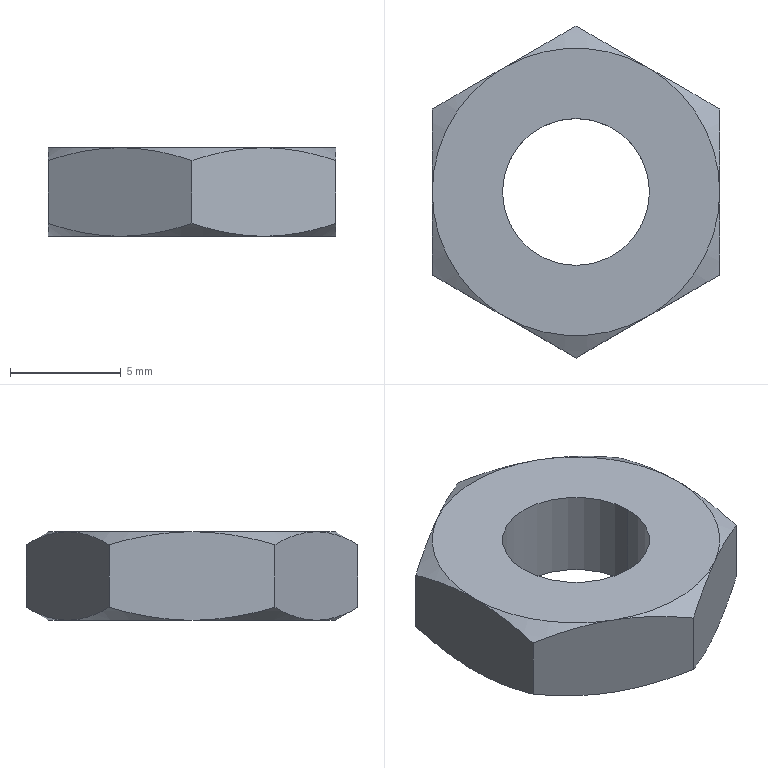Part | SolidWorks | features BaseBody 1 | 1 solid | 22 faces | box 13 x 15.011 x 4 mm | volume 441.798 mm3 | cone 12 | plane 8 | cylinder 2 | commonest cylinder face diameters 6.647 x2
STEP:
#1=CARTESIAN_POINT('',(-3.323,0.,4.));
#2=VERTEX_POINT('',#1);
#3=CARTESIAN_POINT('',(3.323,0.,4.));
#4=VERTEX_POINT('',#3);
#5=CARTESIAN_POINT('',(0.,0.,4.));
#6=DIRECTION('',(0.,0.,1.));
#7=DIRECTION('',(-1.,0.,0.));
#8=AXIS2_PLACEMENT_3D('',#5,#6,#7);
#9=CIRCLE('',#8,3.323);
#10=EDGE_CURVE('',#2,#4,#9,.T.);
#11=ORIENTED_EDGE('',*,*,#10,.T.);
#12=CARTESIAN_POINT('',(3.323,0.,0.));
#13=VERTEX_POINT('',#12);
#14=CARTESIAN_POINT('',(3.323,0.,4.));
#15=DIRECTION('',(0.,0.,-1.));
#16=VECTOR('',#15,1000.);
#17=LINE('',#14,#16);
#18=EDGE_CURVE('',#4,#13,#17,.T.);
#19=ORIENTED_EDGE('',*,*,#18,.T.);
#20=CARTESIAN_POINT('',(-3.323,0.,0.));
#21=VERTEX_POINT('',#20);
#22=CARTESIAN_POINT('',(0.,0.,0.));
#23=DIRECTION('',(0.,0.,1.));
#24=DIRECTION('',(-1.,0.,0.));
#25=AXIS2_PLACEMENT_3D('',#22,#23,#24);
#26=CIRCLE('',#25,3.323);
#27=EDGE_CURVE('',#21,#13,#26,.T.);
#28=ORIENTED_EDGE('',*,*,#27,.F.);
#29=CARTESIAN_POINT('',(-3.323,0.,4.));
#30=DIRECTION('',(0.,0.,-1.));
#31=VECTOR('',#30,1000.);
#32=LINE('',#29,#31);
#33=EDGE_CURVE('',#2,#21,#32,.T.);
#34=ORIENTED_EDGE('',*,*,#33,.F.);
#35=EDGE_LOOP('',(#11,#19,#28,#34));
#36=FACE_OUTER_BOUND('',#35,.T.);
#37=CARTESIAN_POINT('',(0.,0.,4.));
#38=DIRECTION('',(0.,0.,-1.));
#39=DIRECTION('',(-1.,0.,0.));
#40=AXIS2_PLACEMENT_3D('',#37,#38,#39);
#41=CYLINDRICAL_SURFACE('',#40,3.323);
#42=ADVANCED_FACE('',(#36),#41,.F.);
#43=CARTESIAN_POINT('',(-3.25,-5.629,4.));
#44=VERTEX_POINT('',#43);
#45=CARTESIAN_POINT('',(-6.5,0.,4.));
#46=VERTEX_POINT('',#45);
#47=CARTESIAN_POINT('',(0.,0.,4.));
#48=DIRECTION('',(0.,0.,-1.));
#49=DIRECTION('',(-1.,0.,0.));
#50=AXIS2_PLACEMENT_3D('',#47,#48,#49);
#51=CIRCLE('',#50,6.5);
#52=EDGE_CURVE('',#44,#46,#51,.T.);
#53=ORIENTED_EDGE('',*,*,#52,.F.);
#54=CARTESIAN_POINT('',(3.25,-5.629,4.));
#55=VERTEX_POINT('',#54);
#56=CARTESIAN_POINT('',(0.,0.,4.));
#57=DIRECTION('',(0.,0.,-1.));
#58=DIRECTION('',(-1.,0.,0.));
#59=AXIS2_PLACEMENT_3D('',#56,#57,#58);
#60=CIRCLE('',#59,6.5);
#61=EDGE_CURVE('',#55,#44,#60,.T.);
#62=ORIENTED_EDGE('',*,*,#61,.F.);
#63=CARTESIAN_POINT('',(6.5,0.,4.));
#64=VERTEX_POINT('',#63);
#65=CARTESIAN_POINT('',(0.,0.,4.));
#66=DIRECTION('',(0.,0.,-1.));
#67=DIRECTION('',(-1.,0.,0.));
#68=AXIS2_PLACEMENT_3D('',#65,#66,#67);
#69=CIRCLE('',#68,6.5);
#70=EDGE_CURVE('',#64,#55,#69,.T.);
#71=ORIENTED_EDGE('',*,*,#70,.F.);
#72=CARTESIAN_POINT('',(3.25,5.629,4.));
#73=VERTEX_POINT('',#72);
#74=CARTESIAN_POINT('',(0.,0.,4.));
#75=DIRECTION('',(0.,0.,-1.));
#76=DIRECTION('',(-1.,0.,0.));
#77=AXIS2_PLACEMENT_3D('',#74,#75,#76);
#78=CIRCLE('',#77,6.5);
#79=EDGE_CURVE('',#73,#64,#78,.T.);
#80=ORIENTED_EDGE('',*,*,#79,.F.);
#81=CARTESIAN_POINT('',(-3.25,5.629,4.));
#82=VERTEX_POINT('',#81);
#83=CARTESIAN_POINT('',(0.,0.,4.));
#84=DIRECTION('',(0.,0.,-1.));
#85=DIRECTION('',(-1.,0.,0.));
#86=AXIS2_PLACEMENT_3D('',#83,#84,#85);
#87=CIRCLE('',#86,6.5);
#88=EDGE_CURVE('',#82,#73,#87,.T.);
#89=ORIENTED_EDGE('',*,*,#88,.F.);
#90=CARTESIAN_POINT('',(0.,0.,4.));
#91=DIRECTION('',(0.,0.,-1.));
#92=DIRECTION('',(-1.,0.,0.));
#93=AXIS2_PLACEMENT_3D('',#90,#91,#92);
#94=CIRCLE('',#93,6.5);
#95=EDGE_CURVE('',#46,#82,#94,.T.);
#96=ORIENTED_EDGE('',*,*,#95,.F.);
#97=EDGE_LOOP('',(#53,#62,#71,#80,#89,#96));
#98=FACE_OUTER_BOUND('',#97,.T.);
#99=ORIENTED_EDGE('',*,*,#10,.F.);
#100=CARTESIAN_POINT('',(0.,0.,4.));
#101=DIRECTION('',(0.,0.,1.));
#102=DIRECTION('',(-1.,0.,0.));
#103=AXIS2_PLACEMENT_3D('',#100,#101,#102);
#104=CIRCLE('',#103,3.323);
#105=EDGE_CURVE('',#4,#2,#104,.T.);
#106=ORIENTED_EDGE('',*,*,#105,.F.);
#107=EDGE_LOOP('',(#99,#106));
#108=FACE_BOUND('',#107,.T.);
#109=CARTESIAN_POINT('',(6.5,3.753,4.));
#110=DIRECTION('',(0.,0.,-1.));
#111=DIRECTION('',(-1.,0.,0.));
#112=AXIS2_PLACEMENT_3D('',#109,#110,#111);
#113=PLANE('',#112);
#114=ADVANCED_FACE('',(#98,#108),#113,.F.);
#115=CARTESIAN_POINT('',(-6.5,3.753,3.419));
#116=VERTEX_POINT('',#115);
#117=CARTESIAN_POINT('',(-6.5,3.753,3.419));
#118=CARTESIAN_POINT('',(-6.5,2.527,3.773));
#119=CARTESIAN_POINT('',(-6.5,1.281,4.));
#120=CARTESIAN_POINT('',(-6.5,0.,4.));
#121=B_SPLINE_CURVE_WITH_KNOTS('',3,(#117,#118,#119,#120),.UNSPECIFIED.,.F.,.F.,(4,4),(0.,0.003797),.UNSPECIFIED.);
#122=EDGE_CURVE('',#116,#46,#121,.T.);
#123=ORIENTED_EDGE('',*,*,#122,.T.);
#124=ORIENTED_EDGE('',*,*,#95,.T.);
#125=CARTESIAN_POINT('',(-3.25,5.629,4.));
#126=CARTESIAN_POINT('',(-4.359,4.989,4.));
#127=CARTESIAN_POINT('',(-5.438,4.366,3.773));
#128=CARTESIAN_POINT('',(-6.5,3.753,3.419));
#129=B_SPLINE_CURVE_WITH_KNOTS('',3,(#125,#126,#127,#128),.UNSPECIFIED.,.F.,.F.,(4,4),(0.,0.003797),.UNSPECIFIED.);
#130=EDGE_CURVE('',#82,#116,#129,.T.);
#131=ORIENTED_EDGE('',*,*,#130,.T.);
#132=EDGE_LOOP('',(#123,#124,#131));
#133=FACE_OUTER_BOUND('',#132,.T.);
#134=CARTESIAN_POINT('',(0.,0.,3.416));
#135=DIRECTION('',(0.,0.,-1.));
#136=DIRECTION('',(-1.,0.,0.));
#137=AXIS2_PLACEMENT_3D('',#134,#135,#136);
#138=CONICAL_SURFACE('',#137,7.512,1.047);
#139=ADVANCED_FACE('',(#133),#138,.T.);
#140=CARTESIAN_POINT('',(-6.5,-3.753,3.419));
#141=VERTEX_POINT('',#140);
#142=CARTESIAN_POINT('',(-6.5,-3.753,3.419));
#143=CARTESIAN_POINT('',(-5.438,-4.366,3.773));
#144=CARTESIAN_POINT('',(-4.359,-4.989,4.));
#145=CARTESIAN_POINT('',(-3.25,-5.629,4.));
#146=B_SPLINE_CURVE_WITH_KNOTS('',3,(#142,#143,#144,#145),.UNSPECIFIED.,.F.,.F.,(4,4),(0.,0.003797),.UNSPECIFIED.);
#147=EDGE_CURVE('',#141,#44,#146,.T.);
#148=ORIENTED_EDGE('',*,*,#147,.T.);
#149=ORIENTED_EDGE('',*,*,#52,.T.);
#150=CARTESIAN_POINT('',(-6.5,0.,4.));
#151=CARTESIAN_POINT('',(-6.5,-1.281,4.));
#152=CARTESIAN_POINT('',(-6.5,-2.527,3.773));
#153=CARTESIAN_POINT('',(-6.5,-3.753,3.419));
#154=B_SPLINE_CURVE_WITH_KNOTS('',3,(#150,#151,#152,#153),.UNSPECIFIED.,.F.,.F.,(4,4),(0.,0.003797),.UNSPECIFIED.);
#155=EDGE_CURVE('',#46,#141,#154,.T.);
#156=ORIENTED_EDGE('',*,*,#155,.T.);
#157=EDGE_LOOP('',(#148,#149,#156));
#158=FACE_OUTER_BOUND('',#157,.T.);
#159=CARTESIAN_POINT('',(0.,0.,3.416));
#160=DIRECTION('',(0.,0.,-1.));
#161=DIRECTION('',(-1.,0.,0.));
#162=AXIS2_PLACEMENT_3D('',#159,#160,#161);
#163=CONICAL_SURFACE('',#162,7.512,1.047);
#164=ADVANCED_FACE('',(#158),#163,.T.);
#165=CARTESIAN_POINT('',(-0.000000043,-7.506,3.419));
#166=VERTEX_POINT('',#165);
#167=CARTESIAN_POINT('',(-0.000000043,-7.506,3.419));
#168=CARTESIAN_POINT('',(1.062,-6.892,3.773));
#169=CARTESIAN_POINT('',(2.141,-6.27,4.));
#170=CARTESIAN_POINT('',(3.25,-5.629,4.));
#171=B_SPLINE_CURVE_WITH_KNOTS('',3,(#167,#168,#169,#170),.UNSPECIFIED.,.F.,.F.,(4,4),(0.,0.003797),.UNSPECIFIED.);
#172=EDGE_CURVE('',#166,#55,#171,.T.);
#173=ORIENTED_EDGE('',*,*,#172,.T.);
#174=ORIENTED_EDGE('',*,*,#61,.T.);
#175=CARTESIAN_POINT('',(-3.25,-5.629,4.));
#176=CARTESIAN_POINT('',(-2.141,-6.27,4.));
#177=CARTESIAN_POINT('',(-1.062,-6.892,3.773));
#178=CARTESIAN_POINT('',(-0.000000043,-7.506,3.419));
#179=B_SPLINE_CURVE_WITH_KNOTS('',3,(#175,#176,#177,#178),.UNSPECIFIED.,.F.,.F.,(4,4),(0.,0.003797),.UNSPECIFIED.);
#180=EDGE_CURVE('',#44,#166,#179,.T.);
#181=ORIENTED_EDGE('',*,*,#180,.T.);
#182=EDGE_LOOP('',(#173,#174,#181));
#183=FACE_OUTER_BOUND('',#182,.T.);
#184=CARTESIAN_POINT('',(0.,0.,3.416));
#185=DIRECTION('',(0.,0.,-1.));
#186=DIRECTION('',(-1.,0.,0.));
#187=AXIS2_PLACEMENT_3D('',#184,#185,#186);
#188=CONICAL_SURFACE('',#187,7.512,1.047);
#189=ADVANCED_FACE('',(#183),#188,.T.);
#190=CARTESIAN_POINT('',(6.5,-3.753,3.419));
#191=VERTEX_POINT('',#190);
#192=CARTESIAN_POINT('',(6.5,-3.753,3.419));
#193=CARTESIAN_POINT('',(6.5,-2.527,3.773));
#194=CARTESIAN_POINT('',(6.5,-1.281,4.));
#195=CARTESIAN_POINT('',(6.5,0.,4.));
#196=B_SPLINE_CURVE_WITH_KNOTS('',3,(#192,#193,#194,#195),.UNSPECIFIED.,.F.,.F.,(4,4),(0.,0.003797),.UNSPECIFIED.);
#197=EDGE_CURVE('',#191,#64,#196,.T.);
#198=ORIENTED_EDGE('',*,*,#197,.T.);
#199=ORIENTED_EDGE('',*,*,#70,.T.);
#200=CARTESIAN_POINT('',(3.25,-5.629,4.));
#201=CARTESIAN_POINT('',(4.359,-4.989,4.));
#202=CARTESIAN_POINT('',(5.438,-4.366,3.773));
#203=CARTESIAN_POINT('',(6.5,-3.753,3.419));
#204=B_SPLINE_CURVE_WITH_KNOTS('',3,(#200,#201,#202,#203),.UNSPECIFIED.,.F.,.F.,(4,4),(0.,0.003797),.UNSPECIFIED.);
#205=EDGE_CURVE('',#55,#191,#204,.T.);
#206=ORIENTED_EDGE('',*,*,#205,.T.);
#207=EDGE_LOOP('',(#198,#199,#206));
#208=FACE_OUTER_BOUND('',#207,.T.);
#209=CARTESIAN_POINT('',(0.,0.,3.416));
#210=DIRECTION('',(0.,0.,-1.));
#211=DIRECTION('',(-1.,0.,0.));
#212=AXIS2_PLACEMENT_3D('',#209,#210,#211);
#213=CONICAL_SURFACE('',#212,7.512,1.047);
#214=ADVANCED_FACE('',(#208),#213,.T.);
#215=ORIENTED_EDGE('',*,*,#79,.T.);
#216=CARTESIAN_POINT('',(6.5,3.753,3.419));
#217=VERTEX_POINT('',#216);
#218=CARTESIAN_POINT('',(6.5,0.,4.));
#219=CARTESIAN_POINT('',(6.5,1.281,4.));
#220=CARTESIAN_POINT('',(6.5,2.527,3.773));
#221=CARTESIAN_POINT('',(6.5,3.753,3.419));
#222=B_SPLINE_CURVE_WITH_KNOTS('',3,(#218,#219,#220,#221),.UNSPECIFIED.,.F.,.F.,(4,4),(0.,0.003797),.UNSPECIFIED.);
#223=EDGE_CURVE('',#64,#217,#222,.T.);
#224=ORIENTED_EDGE('',*,*,#223,.T.);
#225=CARTESIAN_POINT('',(6.5,3.753,3.419));
#226=CARTESIAN_POINT('',(5.438,4.366,3.773));
#227=CARTESIAN_POINT('',(4.359,4.989,4.));
#228=CARTESIAN_POINT('',(3.25,5.629,4.));
#229=B_SPLINE_CURVE_WITH_KNOTS('',3,(#225,#226,#227,#228),.UNSPECIFIED.,.F.,.F.,(4,4),(0.,0.003797),.UNSPECIFIED.);
#230=EDGE_CURVE('',#217,#73,#229,.T.);
#231=ORIENTED_EDGE('',*,*,#230,.T.);
#232=EDGE_LOOP('',(#215,#224,#231));
#233=FACE_OUTER_BOUND('',#232,.T.);
#234=CARTESIAN_POINT('',(0.,0.,3.416));
#235=DIRECTION('',(0.,0.,-1.));
#236=DIRECTION('',(-1.,0.,0.));
#237=AXIS2_PLACEMENT_3D('',#234,#235,#236);
#238=CONICAL_SURFACE('',#237,7.512,1.047);
#239=ADVANCED_FACE('',(#233),#238,.T.);
#240=CARTESIAN_POINT('',(0.000000043,7.506,3.419));
#241=VERTEX_POINT('',#240);
#242=CARTESIAN_POINT('',(0.000000043,7.506,3.419));
#243=CARTESIAN_POINT('',(-1.062,6.892,3.773));
#244=CARTESIAN_POINT('',(-2.141,6.27,4.));
#245=CARTESIAN_POINT('',(-3.25,5.629,4.));
#246=B_SPLINE_CURVE_WITH_KNOTS('',3,(#242,#243,#244,#245),.UNSPECIFIED.,.F.,.F.,(4,4),(0.,0.003797),.UNSPECIFIED.);
#247=EDGE_CURVE('',#241,#82,#246,.T.);
#248=ORIENTED_EDGE('',*,*,#247,.T.);
#249=ORIENTED_EDGE('',*,*,#88,.T.);
#250=CARTESIAN_POINT('',(3.25,5.629,4.));
#251=CARTESIAN_POINT('',(2.141,6.27,4.));
#252=CARTESIAN_POINT('',(1.062,6.892,3.773));
#253=CARTESIAN_POINT('',(0.000000043,7.506,3.419));
#254=B_SPLINE_CURVE_WITH_KNOTS('',3,(#250,#251,#252,#253),.UNSPECIFIED.,.F.,.F.,(4,4),(0.,0.003797),.UNSPECIFIED.);
#255=EDGE_CURVE('',#73,#241,#254,.T.);
#256=ORIENTED_EDGE('',*,*,#255,.T.);
#257=EDGE_LOOP('',(#248,#249,#256));
#258=FACE_OUTER_BOUND('',#257,.T.);
#259=CARTESIAN_POINT('',(0.,0.,3.416));
#260=DIRECTION('',(0.,0.,-1.));
#261=DIRECTION('',(-1.,0.,0.));
#262=AXIS2_PLACEMENT_3D('',#259,#260,#261);
#263=CONICAL_SURFACE('',#262,7.512,1.047);
#264=ADVANCED_FACE('',(#258),#263,.T.);
#265=ORIENTED_EDGE('',*,*,#18,.F.);
#266=ORIENTED_EDGE('',*,*,#105,.T.);
#267=ORIENTED_EDGE('',*,*,#33,.T.);
#268=CARTESIAN_POINT('',(0.,0.,0.));
#269=DIRECTION('',(0.,0.,1.));
#270=DIRECTION('',(-1.,0.,0.));
#271=AXIS2_PLACEMENT_3D('',#268,#269,#270);
#272=CIRCLE('',#271,3.323);
#273=EDGE_CURVE('',#13,#21,#272,.T.);
#274=ORIENTED_EDGE('',*,*,#273,.F.);
#275=EDGE_LOOP('',(#265,#266,#267,#274));
#276=FACE_OUTER_BOUND('',#275,.T.);
#277=CARTESIAN_POINT('',(0.,0.,4.));
#278=DIRECTION('',(0.,0.,-1.));
#279=DIRECTION('',(-1.,0.,0.));
#280=AXIS2_PLACEMENT_3D('',#277,#278,#279);
#281=CYLINDRICAL_SURFACE('',#280,3.323);
#282=ADVANCED_FACE('',(#276),#281,.F.);
#283=CARTESIAN_POINT('',(-6.5,3.753,0.5806));
#284=VERTEX_POINT('',#283);
#285=CARTESIAN_POINT('',(-6.5,3.753,4.));
#286=DIRECTION('',(0.,0.,1.));
#287=VECTOR('',#286,1000.);
#288=LINE('',#285,#287);
#289=EDGE_CURVE('',#284,#116,#288,.T.);
#290=ORIENTED_EDGE('',*,*,#289,.F.);
#291=CARTESIAN_POINT('',(-6.5,0.,0.));
#292=VERTEX_POINT('',#291);
#293=CARTESIAN_POINT('',(-6.5,0.,0.));
#294=CARTESIAN_POINT('',(-6.5,1.281,0.));
#295=CARTESIAN_POINT('',(-6.5,2.527,0.2266));
#296=CARTESIAN_POINT('',(-6.5,3.753,0.5806));
#297=B_SPLINE_CURVE_WITH_KNOTS('',3,(#293,#294,#295,#296),.UNSPECIFIED.,.F.,.F.,(4,4),(0.,0.003797),.UNSPECIFIED.);
#298=EDGE_CURVE('',#292,#284,#297,.T.);
#299=ORIENTED_EDGE('',*,*,#298,.F.);
#300=CARTESIAN_POINT('',(-6.5,-3.753,0.5806));
#301=VERTEX_POINT('',#300);
#302=CARTESIAN_POINT('',(-6.5,-3.753,0.5806));
#303=CARTESIAN_POINT('',(-6.5,-2.527,0.2266));
#304=CARTESIAN_POINT('',(-6.5,-1.281,0.));
#305=CARTESIAN_POINT('',(-6.5,0.,0.));
#306=B_SPLINE_CURVE_WITH_KNOTS('',3,(#302,#303,#304,#305),.UNSPECIFIED.,.F.,.F.,(4,4),(0.,0.003797),.UNSPECIFIED.);
#307=EDGE_CURVE('',#301,#292,#306,.T.);
#308=ORIENTED_EDGE('',*,*,#307,.F.);
#309=CARTESIAN_POINT('',(-6.5,-3.753,4.));
#310=DIRECTION('',(0.,0.,-1.));
#311=VECTOR('',#310,1000.);
#312=LINE('',#309,#311);
#313=EDGE_CURVE('',#141,#301,#312,.T.);
#314=ORIENTED_EDGE('',*,*,#313,.F.);
#315=ORIENTED_EDGE('',*,*,#155,.F.);
#316=ORIENTED_EDGE('',*,*,#122,.F.);
#317=EDGE_LOOP('',(#290,#299,#308,#314,#315,#316));
#318=FACE_OUTER_BOUND('',#317,.T.);
#319=CARTESIAN_POINT('',(-6.5,3.753,4.));
#320=DIRECTION('',(1.,0.,0.));
#321=DIRECTION('',(0.,1.,0.));
#322=AXIS2_PLACEMENT_3D('',#319,#320,#321);
#323=PLANE('',#322);
#324=ADVANCED_FACE('',(#318),#323,.F.);
#325=CARTESIAN_POINT('',(0.,7.506,0.5806));
#326=VERTEX_POINT('',#325);
#327=CARTESIAN_POINT('',(0.,7.506,4.));
#328=DIRECTION('',(0.,0.,1.));
#329=VECTOR('',#328,1000.);
#330=LINE('',#327,#329);
#331=EDGE_CURVE('',#326,#241,#330,.T.);
#332=ORIENTED_EDGE('',*,*,#331,.F.);
#333=CARTESIAN_POINT('',(-3.25,5.629,0.));
#334=VERTEX_POINT('',#333);
#335=CARTESIAN_POINT('',(-3.25,5.629,0.));
#336=CARTESIAN_POINT('',(-2.141,6.27,0.));
#337=CARTESIAN_POINT('',(-1.062,6.892,0.2266));
#338=CARTESIAN_POINT('',(0.,7.506,0.5806));
#339=B_SPLINE_CURVE_WITH_KNOTS('',3,(#335,#336,#337,#338),.UNSPECIFIED.,.F.,.F.,(4,4),(0.,0.003797),.UNSPECIFIED.);
#340=EDGE_CURVE('',#334,#326,#339,.T.);
#341=ORIENTED_EDGE('',*,*,#340,.F.);
#342=CARTESIAN_POINT('',(-6.5,3.753,0.5806));
#343=CARTESIAN_POINT('',(-5.438,4.366,0.2266));
#344=CARTESIAN_POINT('',(-4.359,4.989,0.));
#345=CARTESIAN_POINT('',(-3.25,5.629,0.));
#346=B_SPLINE_CURVE_WITH_KNOTS('',3,(#342,#343,#344,#345),.UNSPECIFIED.,.F.,.F.,(4,4),(0.,0.003797),.UNSPECIFIED.);
#347=EDGE_CURVE('',#284,#334,#346,.T.);
#348=ORIENTED_EDGE('',*,*,#347,.F.);
#349=ORIENTED_EDGE('',*,*,#289,.T.);
#350=ORIENTED_EDGE('',*,*,#130,.F.);
#351=ORIENTED_EDGE('',*,*,#247,.F.);
#352=EDGE_LOOP('',(#332,#341,#348,#349,#350,#351));
#353=FACE_OUTER_BOUND('',#352,.T.);
#354=CARTESIAN_POINT('',(0.,7.506,4.));
#355=DIRECTION('',(0.5,-0.866,0.));
#356=DIRECTION('',(0.866,0.5,0.));
#357=AXIS2_PLACEMENT_3D('',#354,#355,#356);
#358=PLANE('',#357);
#359=ADVANCED_FACE('',(#353),#358,.F.);
#360=ORIENTED_EDGE('',*,*,#313,.T.);
#361=CARTESIAN_POINT('',(-3.25,-5.629,0.));
#362=VERTEX_POINT('',#361);
#363=CARTESIAN_POINT('',(-3.25,-5.629,0.));
#364=CARTESIAN_POINT('',(-4.359,-4.989,0.));
#365=CARTESIAN_POINT('',(-5.438,-4.366,0.2266));
#366=CARTESIAN_POINT('',(-6.5,-3.753,0.5806));
#367=B_SPLINE_CURVE_WITH_KNOTS('',3,(#363,#364,#365,#366),.UNSPECIFIED.,.F.,.F.,(4,4),(0.,0.003797),.UNSPECIFIED.);
#368=EDGE_CURVE('',#362,#301,#367,.T.);
#369=ORIENTED_EDGE('',*,*,#368,.F.);
#370=CARTESIAN_POINT('',(0.,-7.506,0.5806));
#371=VERTEX_POINT('',#370);
#372=CARTESIAN_POINT('',(0.,-7.506,0.5806));
#373=CARTESIAN_POINT('',(-1.062,-6.892,0.2266));
#374=CARTESIAN_POINT('',(-2.141,-6.27,0.));
#375=CARTESIAN_POINT('',(-3.25,-5.629,0.));
#376=B_SPLINE_CURVE_WITH_KNOTS('',3,(#372,#373,#374,#375),.UNSPECIFIED.,.F.,.F.,(4,4),(0.,0.003797),.UNSPECIFIED.);
#377=EDGE_CURVE('',#371,#362,#376,.T.);
#378=ORIENTED_EDGE('',*,*,#377,.F.);
#379=CARTESIAN_POINT('',(0.,-7.506,4.));
#380=DIRECTION('',(0.,0.,-1.));
#381=VECTOR('',#380,1000.);
#382=LINE('',#379,#381);
#383=EDGE_CURVE('',#166,#371,#382,.T.);
#384=ORIENTED_EDGE('',*,*,#383,.F.);
#385=ORIENTED_EDGE('',*,*,#180,.F.);
#386=ORIENTED_EDGE('',*,*,#147,.F.);
#387=EDGE_LOOP('',(#360,#369,#378,#384,#385,#386));
#388=FACE_OUTER_BOUND('',#387,.T.);
#389=CARTESIAN_POINT('',(-6.5,-3.753,4.));
#390=DIRECTION('',(0.5,0.866,0.));
#391=DIRECTION('',(-0.866,0.5,0.));
#392=AXIS2_PLACEMENT_3D('',#389,#390,#391);
#393=PLANE('',#392);
#394=ADVANCED_FACE('',(#388),#393,.F.);
#395=ORIENTED_EDGE('',*,*,#383,.T.);
#396=CARTESIAN_POINT('',(3.25,-5.629,0.));
#397=VERTEX_POINT('',#396);
#398=CARTESIAN_POINT('',(3.25,-5.629,0.));
#399=CARTESIAN_POINT('',(2.141,-6.27,0.));
#400=CARTESIAN_POINT('',(1.062,-6.892,0.2266));
#401=CARTESIAN_POINT('',(0.,-7.506,0.5806));
#402=B_SPLINE_CURVE_WITH_KNOTS('',3,(#398,#399,#400,#401),.UNSPECIFIED.,.F.,.F.,(4,4),(0.,0.003797),.UNSPECIFIED.);
#403=EDGE_CURVE('',#397,#371,#402,.T.);
#404=ORIENTED_EDGE('',*,*,#403,.F.);
#405=CARTESIAN_POINT('',(6.5,-3.753,0.5806));
#406=VERTEX_POINT('',#405);
#407=CARTESIAN_POINT('',(6.5,-3.753,0.5806));
#408=CARTESIAN_POINT('',(5.438,-4.366,0.2266));
#409=CARTESIAN_POINT('',(4.359,-4.989,0.));
#410=CARTESIAN_POINT('',(3.25,-5.629,0.));
#411=B_SPLINE_CURVE_WITH_KNOTS('',3,(#407,#408,#409,#410),.UNSPECIFIED.,.F.,.F.,(4,4),(0.,0.003797),.UNSPECIFIED.);
#412=EDGE_CURVE('',#406,#397,#411,.T.);
#413=ORIENTED_EDGE('',*,*,#412,.F.);
#414=CARTESIAN_POINT('',(6.5,-3.753,4.));
#415=DIRECTION('',(0.,0.,-1.));
#416=VECTOR('',#415,1000.);
#417=LINE('',#414,#416);
#418=EDGE_CURVE('',#191,#406,#417,.T.);
#419=ORIENTED_EDGE('',*,*,#418,.F.);
#420=ORIENTED_EDGE('',*,*,#205,.F.);
#421=ORIENTED_EDGE('',*,*,#172,.F.);
#422=EDGE_LOOP('',(#395,#404,#413,#419,#420,#421));
#423=FACE_OUTER_BOUND('',#422,.T.);
#424=CARTESIAN_POINT('',(0.,-7.506,4.));
#425=DIRECTION('',(-0.5,0.866,0.));
#426=DIRECTION('',(-0.866,-0.5,0.));
#427=AXIS2_PLACEMENT_3D('',#424,#425,#426);
#428=PLANE('',#427);
#429=ADVANCED_FACE('',(#423),#428,.F.);
#430=ORIENTED_EDGE('',*,*,#418,.T.);
#431=CARTESIAN_POINT('',(6.5,0.,0.));
#432=VERTEX_POINT('',#431);
#433=CARTESIAN_POINT('',(6.5,0.,0.));
#434=CARTESIAN_POINT('',(6.5,-1.281,0.));
#435=CARTESIAN_POINT('',(6.5,-2.527,0.2266));
#436=CARTESIAN_POINT('',(6.5,-3.753,0.5806));
#437=B_SPLINE_CURVE_WITH_KNOTS('',3,(#433,#434,#435,#436),.UNSPECIFIED.,.F.,.F.,(4,4),(0.,0.003797),.UNSPECIFIED.);
#438=EDGE_CURVE('',#432,#406,#437,.T.);
#439=ORIENTED_EDGE('',*,*,#438,.F.);
#440=CARTESIAN_POINT('',(6.5,3.753,0.5806));
#441=VERTEX_POINT('',#440);
#442=CARTESIAN_POINT('',(6.5,3.753,0.5806));
#443=CARTESIAN_POINT('',(6.5,2.527,0.2266));
#444=CARTESIAN_POINT('',(6.5,1.281,0.));
#445=CARTESIAN_POINT('',(6.5,0.,0.));
#446=B_SPLINE_CURVE_WITH_KNOTS('',3,(#442,#443,#444,#445),.UNSPECIFIED.,.F.,.F.,(4,4),(0.,0.003797),.UNSPECIFIED.);
#447=EDGE_CURVE('',#441,#432,#446,.T.);
#448=ORIENTED_EDGE('',*,*,#447,.F.);
#449=CARTESIAN_POINT('',(6.5,3.753,4.));
#450=DIRECTION('',(0.,0.,-1.));
#451=VECTOR('',#450,1000.);
#452=LINE('',#449,#451);
#453=EDGE_CURVE('',#217,#441,#452,.T.);
#454=ORIENTED_EDGE('',*,*,#453,.F.);
#455=ORIENTED_EDGE('',*,*,#223,.F.);
#456=ORIENTED_EDGE('',*,*,#197,.F.);
#457=EDGE_LOOP('',(#430,#439,#448,#454,#455,#456));
#458=FACE_OUTER_BOUND('',#457,.T.);
#459=CARTESIAN_POINT('',(6.5,-3.753,4.));
#460=DIRECTION('',(-1.,0.,0.));
#461=DIRECTION('',(0.,-1.,0.));
#462=AXIS2_PLACEMENT_3D('',#459,#460,#461);
#463=PLANE('',#462);
#464=ADVANCED_FACE('',(#458),#463,.F.);
#465=ORIENTED_EDGE('',*,*,#453,.T.);
#466=CARTESIAN_POINT('',(3.25,5.629,0.));
#467=VERTEX_POINT('',#466);
#468=CARTESIAN_POINT('',(3.25,5.629,0.));
#469=CARTESIAN_POINT('',(4.359,4.989,0.));
#470=CARTESIAN_POINT('',(5.438,4.366,0.2266));
#471=CARTESIAN_POINT('',(6.5,3.753,0.5806));
#472=B_SPLINE_CURVE_WITH_KNOTS('',3,(#468,#469,#470,#471),.UNSPECIFIED.,.F.,.F.,(4,4),(0.,0.003797),.UNSPECIFIED.);
#473=EDGE_CURVE('',#467,#441,#472,.T.);
#474=ORIENTED_EDGE('',*,*,#473,.F.);
#475=CARTESIAN_POINT('',(0.,7.506,0.5806));
#476=CARTESIAN_POINT('',(1.062,6.892,0.2266));
#477=CARTESIAN_POINT('',(2.141,6.27,0.));
#478=CARTESIAN_POINT('',(3.25,5.629,0.));
#479=B_SPLINE_CURVE_WITH_KNOTS('',3,(#475,#476,#477,#478),.UNSPECIFIED.,.F.,.F.,(4,4),(0.,0.003797),.UNSPECIFIED.);
#480=EDGE_CURVE('',#326,#467,#479,.T.);
#481=ORIENTED_EDGE('',*,*,#480,.F.);
#482=ORIENTED_EDGE('',*,*,#331,.T.);
#483=ORIENTED_EDGE('',*,*,#255,.F.);
#484=ORIENTED_EDGE('',*,*,#230,.F.);
#485=EDGE_LOOP('',(#465,#474,#481,#482,#483,#484));
#486=FACE_OUTER_BOUND('',#485,.T.);
#487=CARTESIAN_POINT('',(6.5,3.753,4.));
#488=DIRECTION('',(-0.5,-0.866,0.));
#489=DIRECTION('',(0.866,-0.5,0.));
#490=AXIS2_PLACEMENT_3D('',#487,#488,#489);
#491=PLANE('',#490);
#492=ADVANCED_FACE('',(#486),#491,.F.);
#493=CARTESIAN_POINT('',(0.,0.,0.));
#494=DIRECTION('',(0.,0.,-1.));
#495=DIRECTION('',(1.,0.,0.));
#496=AXIS2_PLACEMENT_3D('',#493,#494,#495);
#497=CIRCLE('',#496,6.5);
#498=EDGE_CURVE('',#432,#397,#497,.T.);
#499=ORIENTED_EDGE('',*,*,#498,.T.);
#500=CARTESIAN_POINT('',(0.,0.,0.));
#501=DIRECTION('',(0.,0.,-1.));
#502=DIRECTION('',(1.,0.,0.));
#503=AXIS2_PLACEMENT_3D('',#500,#501,#502);
#504=CIRCLE('',#503,6.5);
#505=EDGE_CURVE('',#397,#362,#504,.T.);
#506=ORIENTED_EDGE('',*,*,#505,.T.);
#507=CARTESIAN_POINT('',(0.,0.,0.));
#508=DIRECTION('',(0.,0.,-1.));
#509=DIRECTION('',(1.,0.,0.));
#510=AXIS2_PLACEMENT_3D('',#507,#508,#509);
#511=CIRCLE('',#510,6.5);
#512=EDGE_CURVE('',#362,#292,#511,.T.);
#513=ORIENTED_EDGE('',*,*,#512,.T.);
#514=CARTESIAN_POINT('',(0.,0.,0.));
#515=DIRECTION('',(0.,0.,-1.));
#516=DIRECTION('',(1.,0.,0.));
#517=AXIS2_PLACEMENT_3D('',#514,#515,#516);
#518=CIRCLE('',#517,6.5);
#519=EDGE_CURVE('',#292,#334,#518,.T.);
#520=ORIENTED_EDGE('',*,*,#519,.T.);
#521=CARTESIAN_POINT('',(0.,0.,0.));
#522=DIRECTION('',(0.,0.,-1.));
#523=DIRECTION('',(1.,0.,0.));
#524=AXIS2_PLACEMENT_3D('',#521,#522,#523);
#525=CIRCLE('',#524,6.5);
#526=EDGE_CURVE('',#334,#467,#525,.T.);
#527=ORIENTED_EDGE('',*,*,#526,.T.);
#528=CARTESIAN_POINT('',(0.,0.,0.));
#529=DIRECTION('',(0.,0.,-1.));
#530=DIRECTION('',(1.,0.,0.));
#531=AXIS2_PLACEMENT_3D('',#528,#529,#530);
#532=CIRCLE('',#531,6.5);
#533=EDGE_CURVE('',#467,#432,#532,.T.);
#534=ORIENTED_EDGE('',*,*,#533,.T.);
#535=EDGE_LOOP('',(#499,#506,#513,#520,#527,#534));
#536=FACE_OUTER_BOUND('',#535,.T.);
#537=ORIENTED_EDGE('',*,*,#27,.T.);
#538=ORIENTED_EDGE('',*,*,#273,.T.);
#539=EDGE_LOOP('',(#537,#538));
#540=FACE_BOUND('',#539,.T.);
#541=CARTESIAN_POINT('',(6.5,3.753,0.));
#542=DIRECTION('',(0.,0.,-1.));
#543=DIRECTION('',(-1.,0.,0.));
#544=AXIS2_PLACEMENT_3D('',#541,#542,#543);
#545=PLANE('',#544);
#546=ADVANCED_FACE('',(#536,#540),#545,.T.);
#547=ORIENTED_EDGE('',*,*,#347,.T.);
#548=ORIENTED_EDGE('',*,*,#519,.F.);
#549=ORIENTED_EDGE('',*,*,#298,.T.);
#550=EDGE_LOOP('',(#547,#548,#549));
#551=FACE_OUTER_BOUND('',#550,.T.);
#552=CARTESIAN_POINT('',(0.,0.,0.584));
#553=DIRECTION('',(0.,0.,1.));
#554=DIRECTION('',(1.,0.,0.));
#555=AXIS2_PLACEMENT_3D('',#552,#553,#554);
#556=CONICAL_SURFACE('',#555,7.512,1.047);
#557=ADVANCED_FACE('',(#551),#556,.T.);
#558=ORIENTED_EDGE('',*,*,#512,.F.);
#559=ORIENTED_EDGE('',*,*,#368,.T.);
#560=ORIENTED_EDGE('',*,*,#307,.T.);
#561=EDGE_LOOP('',(#558,#559,#560));
#562=FACE_OUTER_BOUND('',#561,.T.);
#563=CARTESIAN_POINT('',(0.,0.,0.584));
#564=DIRECTION('',(0.,0.,1.));
#565=DIRECTION('',(1.,0.,0.));
#566=AXIS2_PLACEMENT_3D('',#563,#564,#565);
#567=CONICAL_SURFACE('',#566,7.512,1.047);
#568=ADVANCED_FACE('',(#562),#567,.T.);
#569=ORIENTED_EDGE('',*,*,#480,.T.);
#570=ORIENTED_EDGE('',*,*,#526,.F.);
#571=ORIENTED_EDGE('',*,*,#340,.T.);
#572=EDGE_LOOP('',(#569,#570,#571));
#573=FACE_OUTER_BOUND('',#572,.T.);
#574=CARTESIAN_POINT('',(0.,0.,0.584));
#575=DIRECTION('',(0.,0.,1.));
#576=DIRECTION('',(1.,0.,0.));
#577=AXIS2_PLACEMENT_3D('',#574,#575,#576);
#578=CONICAL_SURFACE('',#577,7.512,1.047);
#579=ADVANCED_FACE('',(#573),#578,.T.);
#580=ORIENTED_EDGE('',*,*,#505,.F.);
#581=ORIENTED_EDGE('',*,*,#403,.T.);
#582=ORIENTED_EDGE('',*,*,#377,.T.);
#583=EDGE_LOOP('',(#580,#581,#582));
#584=FACE_OUTER_BOUND('',#583,.T.);
#585=CARTESIAN_POINT('',(0.,0.,0.584));
#586=DIRECTION('',(0.,0.,1.));
#587=DIRECTION('',(1.,0.,0.));
#588=AXIS2_PLACEMENT_3D('',#585,#586,#587);
#589=CONICAL_SURFACE('',#588,7.512,1.047);
#590=ADVANCED_FACE('',(#584),#589,.T.);
#591=ORIENTED_EDGE('',*,*,#498,.F.);
#592=ORIENTED_EDGE('',*,*,#438,.T.);
#593=ORIENTED_EDGE('',*,*,#412,.T.);
#594=EDGE_LOOP('',(#591,#592,#593));
#595=FACE_OUTER_BOUND('',#594,.T.);
#596=CARTESIAN_POINT('',(0.,0.,0.584));
#597=DIRECTION('',(0.,0.,1.));
#598=DIRECTION('',(1.,0.,0.));
#599=AXIS2_PLACEMENT_3D('',#596,#597,#598);
#600=CONICAL_SURFACE('',#599,7.512,1.047);
#601=ADVANCED_FACE('',(#595),#600,.T.);
#602=ORIENTED_EDGE('',*,*,#447,.T.);
#603=ORIENTED_EDGE('',*,*,#533,.F.);
#604=ORIENTED_EDGE('',*,*,#473,.T.);
#605=EDGE_LOOP('',(#602,#603,#604));
#606=FACE_OUTER_BOUND('',#605,.T.);
#607=CARTESIAN_POINT('',(0.,0.,0.584));
#608=DIRECTION('',(0.,0.,1.));
#609=DIRECTION('',(1.,0.,0.));
#610=AXIS2_PLACEMENT_3D('',#607,#608,#609);
#611=CONICAL_SURFACE('',#610,7.512,1.047);
#612=ADVANCED_FACE('',(#606),#611,.T.);
#613=CLOSED_SHELL('',(#42,#114,#139,#164,#189,#214,#239,#264,#282,#324,#359,#394,#429,#464,#492,#546,#557,#568,#579,#590,#601,#612));
#614=MANIFOLD_SOLID_BREP('',#613);
#615=CARTESIAN_POINT('',(0.,0.,0.));
#616=DIRECTION('',(0.,0.,1.));
#617=DIRECTION('',(1.,0.,0.));
#618=AXIS2_PLACEMENT_3D('',#615,#616,#617);
#619=(LENGTH_UNIT()NAMED_UNIT(*)SI_UNIT(.MILLI.,.METRE.));
#620=UNCERTAINTY_MEASURE_WITH_UNIT(LENGTH_MEASURE(0.00001),#619,'','');
#621=(NAMED_UNIT(*)PLANE_ANGLE_UNIT()SI_UNIT($,.RADIAN.));
#622=(NAMED_UNIT(*)SI_UNIT($,.STERADIAN.)SOLID_ANGLE_UNIT());
#623=(GEOMETRIC_REPRESENTATION_CONTEXT(3)GLOBAL_UNCERTAINTY_ASSIGNED_CONTEXT((#620))GLOBAL_UNIT_ASSIGNED_CONTEXT((#619,#621,#622))REPRESENTATION_CONTEXT('',''));
#624=ADVANCED_BREP_SHAPE_REPRESENTATION('',(#614,#618),#623);